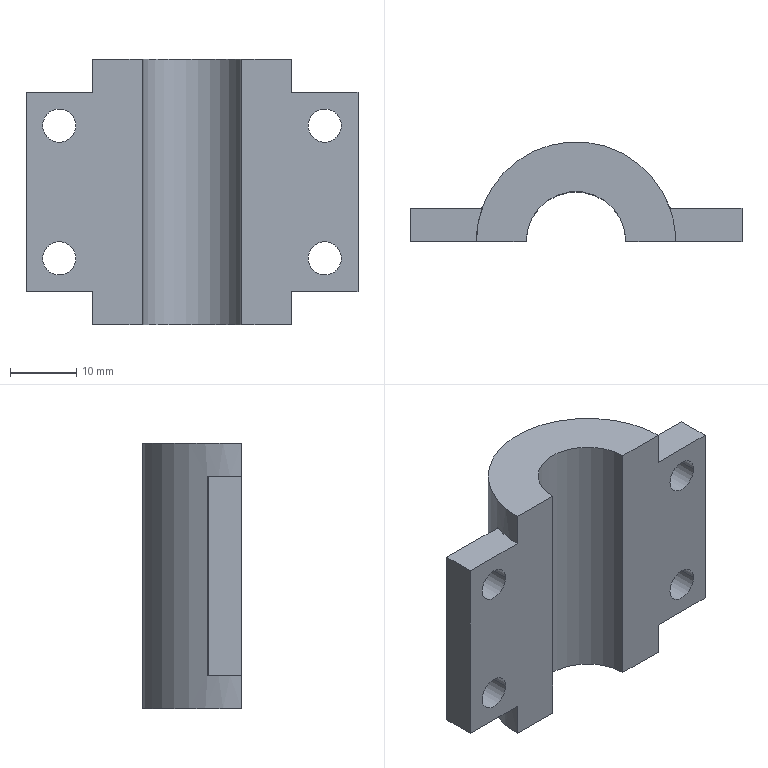Part | SolidWorks | features BaseBody 1 | 1 solid | 28 faces | box 50 x 15 x 40 mm | volume 13295 mm3 | cylinder 16 | plane 12 | commonest cylinder face diameters 5 x8 0.5 x4 30 x3 15 x1
STEP:
#1=CARTESIAN_POINT('',(-17.5,0.,10.));
#2=VERTEX_POINT('',#1);
#3=CARTESIAN_POINT('',(-22.5,0.,10.));
#4=VERTEX_POINT('',#3);
#5=CARTESIAN_POINT('',(-20.,0.,10.));
#6=DIRECTION('',(0.,1.,0.));
#7=DIRECTION('',(-1.,0.,0.));
#8=AXIS2_PLACEMENT_3D('',#5,#6,#7);
#9=CIRCLE('',#8,2.5);
#10=EDGE_CURVE('',#2,#4,#9,.T.);
#11=ORIENTED_EDGE('',*,*,#10,.F.);
#12=CARTESIAN_POINT('',(-17.5,5.,10.));
#13=VERTEX_POINT('',#12);
#14=CARTESIAN_POINT('',(-17.5,5.,10.));
#15=DIRECTION('',(0.,1.,0.));
#16=VECTOR('',#15,1000.);
#17=LINE('',#14,#16);
#18=EDGE_CURVE('',#2,#13,#17,.T.);
#19=ORIENTED_EDGE('',*,*,#18,.T.);
#20=CARTESIAN_POINT('',(-22.5,5.,10.));
#21=VERTEX_POINT('',#20);
#22=CARTESIAN_POINT('',(-20.,5.,10.));
#23=DIRECTION('',(0.,-1.,0.));
#24=DIRECTION('',(-1.,0.,0.));
#25=AXIS2_PLACEMENT_3D('',#22,#23,#24);
#26=CIRCLE('',#25,2.5);
#27=EDGE_CURVE('',#21,#13,#26,.T.);
#28=ORIENTED_EDGE('',*,*,#27,.F.);
#29=CARTESIAN_POINT('',(-22.5,5.,10.));
#30=DIRECTION('',(0.,1.,0.));
#31=VECTOR('',#30,1000.);
#32=LINE('',#29,#31);
#33=EDGE_CURVE('',#4,#21,#32,.T.);
#34=ORIENTED_EDGE('',*,*,#33,.F.);
#35=EDGE_LOOP('',(#11,#19,#28,#34));
#36=FACE_OUTER_BOUND('',#35,.T.);
#37=CARTESIAN_POINT('',(-20.,5.,10.));
#38=DIRECTION('',(0.,1.,0.));
#39=DIRECTION('',(-1.,0.,0.));
#40=AXIS2_PLACEMENT_3D('',#37,#38,#39);
#41=CYLINDRICAL_SURFACE('',#40,2.5);
#42=ADVANCED_FACE('',(#36),#41,.F.);
#43=CARTESIAN_POINT('',(22.5,0.,10.));
#44=VERTEX_POINT('',#43);
#45=CARTESIAN_POINT('',(17.5,0.,10.));
#46=VERTEX_POINT('',#45);
#47=CARTESIAN_POINT('',(20.,0.,10.));
#48=DIRECTION('',(0.,1.,0.));
#49=DIRECTION('',(-1.,0.,0.));
#50=AXIS2_PLACEMENT_3D('',#47,#48,#49);
#51=CIRCLE('',#50,2.5);
#52=EDGE_CURVE('',#44,#46,#51,.T.);
#53=ORIENTED_EDGE('',*,*,#52,.F.);
#54=CARTESIAN_POINT('',(22.5,5.,10.));
#55=VERTEX_POINT('',#54);
#56=CARTESIAN_POINT('',(22.5,5.,10.));
#57=DIRECTION('',(0.,1.,0.));
#58=VECTOR('',#57,1000.);
#59=LINE('',#56,#58);
#60=EDGE_CURVE('',#44,#55,#59,.T.);
#61=ORIENTED_EDGE('',*,*,#60,.T.);
#62=CARTESIAN_POINT('',(17.5,5.,10.));
#63=VERTEX_POINT('',#62);
#64=CARTESIAN_POINT('',(20.,5.,10.));
#65=DIRECTION('',(0.,-1.,0.));
#66=DIRECTION('',(-1.,0.,0.));
#67=AXIS2_PLACEMENT_3D('',#64,#65,#66);
#68=CIRCLE('',#67,2.5);
#69=EDGE_CURVE('',#63,#55,#68,.T.);
#70=ORIENTED_EDGE('',*,*,#69,.F.);
#71=CARTESIAN_POINT('',(17.5,5.,10.));
#72=DIRECTION('',(0.,1.,0.));
#73=VECTOR('',#72,1000.);
#74=LINE('',#71,#73);
#75=EDGE_CURVE('',#46,#63,#74,.T.);
#76=ORIENTED_EDGE('',*,*,#75,.F.);
#77=EDGE_LOOP('',(#53,#61,#70,#76));
#78=FACE_OUTER_BOUND('',#77,.T.);
#79=CARTESIAN_POINT('',(20.,5.,10.));
#80=DIRECTION('',(0.,1.,0.));
#81=DIRECTION('',(-1.,0.,0.));
#82=AXIS2_PLACEMENT_3D('',#79,#80,#81);
#83=CYLINDRICAL_SURFACE('',#82,2.5);
#84=ADVANCED_FACE('',(#78),#83,.F.);
#85=CARTESIAN_POINT('',(22.5,0.,30.));
#86=VERTEX_POINT('',#85);
#87=CARTESIAN_POINT('',(17.5,0.,30.));
#88=VERTEX_POINT('',#87);
#89=CARTESIAN_POINT('',(20.,0.,30.));
#90=DIRECTION('',(0.,1.,0.));
#91=DIRECTION('',(-1.,0.,0.));
#92=AXIS2_PLACEMENT_3D('',#89,#90,#91);
#93=CIRCLE('',#92,2.5);
#94=EDGE_CURVE('',#86,#88,#93,.T.);
#95=ORIENTED_EDGE('',*,*,#94,.F.);
#96=CARTESIAN_POINT('',(22.5,5.,30.));
#97=VERTEX_POINT('',#96);
#98=CARTESIAN_POINT('',(22.5,5.,30.));
#99=DIRECTION('',(0.,1.,0.));
#100=VECTOR('',#99,1000.);
#101=LINE('',#98,#100);
#102=EDGE_CURVE('',#86,#97,#101,.T.);
#103=ORIENTED_EDGE('',*,*,#102,.T.);
#104=CARTESIAN_POINT('',(17.5,5.,30.));
#105=VERTEX_POINT('',#104);
#106=CARTESIAN_POINT('',(20.,5.,30.));
#107=DIRECTION('',(0.,-1.,0.));
#108=DIRECTION('',(-1.,0.,0.));
#109=AXIS2_PLACEMENT_3D('',#106,#107,#108);
#110=CIRCLE('',#109,2.5);
#111=EDGE_CURVE('',#105,#97,#110,.T.);
#112=ORIENTED_EDGE('',*,*,#111,.F.);
#113=CARTESIAN_POINT('',(17.5,5.,30.));
#114=DIRECTION('',(0.,1.,0.));
#115=VECTOR('',#114,1000.);
#116=LINE('',#113,#115);
#117=EDGE_CURVE('',#88,#105,#116,.T.);
#118=ORIENTED_EDGE('',*,*,#117,.F.);
#119=EDGE_LOOP('',(#95,#103,#112,#118));
#120=FACE_OUTER_BOUND('',#119,.T.);
#121=CARTESIAN_POINT('',(20.,5.,30.));
#122=DIRECTION('',(0.,1.,0.));
#123=DIRECTION('',(-1.,0.,0.));
#124=AXIS2_PLACEMENT_3D('',#121,#122,#123);
#125=CYLINDRICAL_SURFACE('',#124,2.5);
#126=ADVANCED_FACE('',(#120),#125,.F.);
#127=CARTESIAN_POINT('',(-17.5,0.,30.));
#128=VERTEX_POINT('',#127);
#129=CARTESIAN_POINT('',(-22.5,0.,30.));
#130=VERTEX_POINT('',#129);
#131=CARTESIAN_POINT('',(-20.,0.,30.));
#132=DIRECTION('',(0.,1.,0.));
#133=DIRECTION('',(-1.,0.,0.));
#134=AXIS2_PLACEMENT_3D('',#131,#132,#133);
#135=CIRCLE('',#134,2.5);
#136=EDGE_CURVE('',#128,#130,#135,.T.);
#137=ORIENTED_EDGE('',*,*,#136,.F.);
#138=CARTESIAN_POINT('',(-17.5,5.,30.));
#139=VERTEX_POINT('',#138);
#140=CARTESIAN_POINT('',(-17.5,5.,30.));
#141=DIRECTION('',(0.,1.,0.));
#142=VECTOR('',#141,1000.);
#143=LINE('',#140,#142);
#144=EDGE_CURVE('',#128,#139,#143,.T.);
#145=ORIENTED_EDGE('',*,*,#144,.T.);
#146=CARTESIAN_POINT('',(-22.5,5.,30.));
#147=VERTEX_POINT('',#146);
#148=CARTESIAN_POINT('',(-20.,5.,30.));
#149=DIRECTION('',(0.,-1.,0.));
#150=DIRECTION('',(-1.,0.,0.));
#151=AXIS2_PLACEMENT_3D('',#148,#149,#150);
#152=CIRCLE('',#151,2.5);
#153=EDGE_CURVE('',#147,#139,#152,.T.);
#154=ORIENTED_EDGE('',*,*,#153,.F.);
#155=CARTESIAN_POINT('',(-22.5,5.,30.));
#156=DIRECTION('',(0.,1.,0.));
#157=VECTOR('',#156,1000.);
#158=LINE('',#155,#157);
#159=EDGE_CURVE('',#130,#147,#158,.T.);
#160=ORIENTED_EDGE('',*,*,#159,.F.);
#161=EDGE_LOOP('',(#137,#145,#154,#160));
#162=FACE_OUTER_BOUND('',#161,.T.);
#163=CARTESIAN_POINT('',(-20.,5.,30.));
#164=DIRECTION('',(0.,1.,0.));
#165=DIRECTION('',(-1.,0.,0.));
#166=AXIS2_PLACEMENT_3D('',#163,#164,#165);
#167=CYLINDRICAL_SURFACE('',#166,2.5);
#168=ADVANCED_FACE('',(#162),#167,.F.);
#169=CARTESIAN_POINT('',(-14.083,5.164,5.));
#170=VERTEX_POINT('',#169);
#171=CARTESIAN_POINT('',(-14.175,5.045,5.));
#172=VERTEX_POINT('',#171);
#173=CARTESIAN_POINT('',(-14.318,5.25,5.));
#174=DIRECTION('',(0.,0.,-1.));
#175=DIRECTION('',(0.5726,-0.8198,0.));
#176=AXIS2_PLACEMENT_3D('',#173,#174,#175);
#177=CIRCLE('',#176,0.25);
#178=EDGE_CURVE('',#170,#172,#177,.T.);
#179=ORIENTED_EDGE('',*,*,#178,.T.);
#180=CARTESIAN_POINT('',(-14.175,5.045,35.));
#181=VERTEX_POINT('',#180);
#182=CARTESIAN_POINT('',(-14.175,5.045,0.));
#183=DIRECTION('',(0.,0.,1.));
#184=VECTOR('',#183,1000.);
#185=LINE('',#182,#184);
#186=EDGE_CURVE('',#172,#181,#185,.T.);
#187=ORIENTED_EDGE('',*,*,#186,.T.);
#188=CARTESIAN_POINT('',(-14.083,5.164,35.));
#189=VERTEX_POINT('',#188);
#190=CARTESIAN_POINT('',(-14.318,5.25,35.));
#191=DIRECTION('',(0.,0.,1.));
#192=DIRECTION('',(0.5726,-0.8198,0.));
#193=AXIS2_PLACEMENT_3D('',#190,#191,#192);
#194=CIRCLE('',#193,0.25);
#195=EDGE_CURVE('',#181,#189,#194,.T.);
#196=ORIENTED_EDGE('',*,*,#195,.T.);
#197=CARTESIAN_POINT('',(-14.083,5.164,0.));
#198=DIRECTION('',(0.,0.,-1.));
#199=VECTOR('',#198,1000.);
#200=LINE('',#197,#199);
#201=EDGE_CURVE('',#189,#170,#200,.T.);
#202=ORIENTED_EDGE('',*,*,#201,.T.);
#203=EDGE_LOOP('',(#179,#187,#196,#202));
#204=FACE_OUTER_BOUND('',#203,.T.);
#205=CARTESIAN_POINT('',(-14.318,5.25,0.));
#206=DIRECTION('',(0.,0.,1.));
#207=DIRECTION('',(0.5726,-0.8198,0.));
#208=AXIS2_PLACEMENT_3D('',#205,#206,#207);
#209=CYLINDRICAL_SURFACE('',#208,0.25);
#210=ADVANCED_FACE('',(#204),#209,.F.);
#211=CARTESIAN_POINT('',(14.142,5.,40.));
#212=VERTEX_POINT('',#211);
#213=CARTESIAN_POINT('',(-15.,0.,40.));
#214=VERTEX_POINT('',#213);
#215=CARTESIAN_POINT('',(0.,0.,40.));
#216=DIRECTION('',(0.,0.,1.));
#217=DIRECTION('',(0.9428,-0.3333,0.));
#218=AXIS2_PLACEMENT_3D('',#215,#216,#217);
#219=CIRCLE('',#218,15.);
#220=EDGE_CURVE('',#212,#214,#219,.T.);
#221=ORIENTED_EDGE('',*,*,#220,.F.);
#222=CARTESIAN_POINT('',(14.142,5.,35.));
#223=VERTEX_POINT('',#222);
#224=CARTESIAN_POINT('',(14.142,5.,0.));
#225=DIRECTION('',(0.,0.,-1.));
#226=VECTOR('',#225,1000.);
#227=LINE('',#224,#226);
#228=EDGE_CURVE('',#212,#223,#227,.T.);
#229=ORIENTED_EDGE('',*,*,#228,.T.);
#230=CARTESIAN_POINT('',(14.083,5.164,35.));
#231=VERTEX_POINT('',#230);
#232=CARTESIAN_POINT('',(0.,0.,35.));
#233=DIRECTION('',(0.,0.,1.));
#234=DIRECTION('',(0.9428,0.3333,0.));
#235=AXIS2_PLACEMENT_3D('',#232,#233,#234);
#236=CIRCLE('',#235,15.);
#237=EDGE_CURVE('',#223,#231,#236,.T.);
#238=ORIENTED_EDGE('',*,*,#237,.T.);
#239=CARTESIAN_POINT('',(14.083,5.164,5.));
#240=VERTEX_POINT('',#239);
#241=CARTESIAN_POINT('',(14.083,5.164,0.));
#242=DIRECTION('',(0.,0.,1.));
#243=VECTOR('',#242,1000.);
#244=LINE('',#241,#243);
#245=EDGE_CURVE('',#240,#231,#244,.T.);
#246=ORIENTED_EDGE('',*,*,#245,.F.);
#247=CARTESIAN_POINT('',(14.142,5.,5.));
#248=VERTEX_POINT('',#247);
#249=CARTESIAN_POINT('',(0.,0.,5.));
#250=DIRECTION('',(0.,0.,-1.));
#251=DIRECTION('',(0.9428,0.3333,0.));
#252=AXIS2_PLACEMENT_3D('',#249,#250,#251);
#253=CIRCLE('',#252,15.);
#254=EDGE_CURVE('',#240,#248,#253,.T.);
#255=ORIENTED_EDGE('',*,*,#254,.T.);
#256=CARTESIAN_POINT('',(14.142,5.,0.));
#257=VERTEX_POINT('',#256);
#258=CARTESIAN_POINT('',(14.142,5.,0.));
#259=DIRECTION('',(0.,0.,-1.));
#260=VECTOR('',#259,1000.);
#261=LINE('',#258,#260);
#262=EDGE_CURVE('',#248,#257,#261,.T.);
#263=ORIENTED_EDGE('',*,*,#262,.T.);
#264=CARTESIAN_POINT('',(-15.,0.,0.));
#265=VERTEX_POINT('',#264);
#266=CARTESIAN_POINT('',(0.,0.,0.));
#267=DIRECTION('',(0.,0.,-1.));
#268=DIRECTION('',(-1.,0.,0.));
#269=AXIS2_PLACEMENT_3D('',#266,#267,#268);
#270=CIRCLE('',#269,15.);
#271=EDGE_CURVE('',#265,#257,#270,.T.);
#272=ORIENTED_EDGE('',*,*,#271,.F.);
#273=CARTESIAN_POINT('',(-15.,0.,5.));
#274=VERTEX_POINT('',#273);
#275=CARTESIAN_POINT('',(-15.,0.,5.));
#276=DIRECTION('',(0.,0.,-1.));
#277=VECTOR('',#276,1000.);
#278=LINE('',#275,#277);
#279=EDGE_CURVE('',#274,#265,#278,.T.);
#280=ORIENTED_EDGE('',*,*,#279,.F.);
#281=CARTESIAN_POINT('',(0.,0.,5.));
#282=DIRECTION('',(0.,0.,-1.));
#283=DIRECTION('',(0.9428,0.3333,0.));
#284=AXIS2_PLACEMENT_3D('',#281,#282,#283);
#285=CIRCLE('',#284,15.);
#286=EDGE_CURVE('',#274,#170,#285,.T.);
#287=ORIENTED_EDGE('',*,*,#286,.T.);
#288=ORIENTED_EDGE('',*,*,#201,.F.);
#289=CARTESIAN_POINT('',(-15.,0.,35.));
#290=VERTEX_POINT('',#289);
#291=CARTESIAN_POINT('',(0.,0.,35.));
#292=DIRECTION('',(0.,0.,1.));
#293=DIRECTION('',(0.9428,0.3333,0.));
#294=AXIS2_PLACEMENT_3D('',#291,#292,#293);
#295=CIRCLE('',#294,15.);
#296=EDGE_CURVE('',#189,#290,#295,.T.);
#297=ORIENTED_EDGE('',*,*,#296,.T.);
#298=CARTESIAN_POINT('',(-15.,0.,40.));
#299=DIRECTION('',(0.,0.,-1.));
#300=VECTOR('',#299,1000.);
#301=LINE('',#298,#300);
#302=EDGE_CURVE('',#214,#290,#301,.T.);
#303=ORIENTED_EDGE('',*,*,#302,.F.);
#304=EDGE_LOOP('',(#221,#229,#238,#246,#255,#263,#272,#280,#287,#288,#297,#303));
#305=FACE_OUTER_BOUND('',#304,.T.);
#306=CARTESIAN_POINT('',(0.,0.,0.));
#307=DIRECTION('',(0.,0.,-1.));
#308=DIRECTION('',(0.9428,0.3333,0.));
#309=AXIS2_PLACEMENT_3D('',#306,#307,#308);
#310=CYLINDRICAL_SURFACE('',#309,15.);
#311=ADVANCED_FACE('',(#305),#310,.T.);
#312=ORIENTED_EDGE('',*,*,#228,.F.);
#313=CARTESIAN_POINT('',(15.,0.,40.));
#314=VERTEX_POINT('',#313);
#315=CARTESIAN_POINT('',(0.,0.,40.));
#316=DIRECTION('',(0.,0.,1.));
#317=DIRECTION('',(0.9428,-0.3333,0.));
#318=AXIS2_PLACEMENT_3D('',#315,#316,#317);
#319=CIRCLE('',#318,15.);
#320=EDGE_CURVE('',#314,#212,#319,.T.);
#321=ORIENTED_EDGE('',*,*,#320,.F.);
#322=CARTESIAN_POINT('',(15.,0.,35.));
#323=VERTEX_POINT('',#322);
#324=CARTESIAN_POINT('',(15.,0.,40.));
#325=DIRECTION('',(0.,0.,1.));
#326=VECTOR('',#325,1000.);
#327=LINE('',#324,#326);
#328=EDGE_CURVE('',#323,#314,#327,.T.);
#329=ORIENTED_EDGE('',*,*,#328,.F.);
#330=CARTESIAN_POINT('',(0.,0.,35.));
#331=DIRECTION('',(0.,0.,1.));
#332=DIRECTION('',(0.9428,0.3333,0.));
#333=AXIS2_PLACEMENT_3D('',#330,#331,#332);
#334=CIRCLE('',#333,15.);
#335=EDGE_CURVE('',#323,#223,#334,.T.);
#336=ORIENTED_EDGE('',*,*,#335,.T.);
#337=EDGE_LOOP('',(#312,#321,#329,#336));
#338=FACE_OUTER_BOUND('',#337,.T.);
#339=CARTESIAN_POINT('',(0.,0.,0.));
#340=DIRECTION('',(0.,0.,-1.));
#341=DIRECTION('',(0.9428,0.3333,0.));
#342=AXIS2_PLACEMENT_3D('',#339,#340,#341);
#343=CYLINDRICAL_SURFACE('',#342,15.);
#344=ADVANCED_FACE('',(#338),#343,.T.);
#345=CARTESIAN_POINT('',(14.175,5.045,35.));
#346=VERTEX_POINT('',#345);
#347=CARTESIAN_POINT('',(14.318,5.25,35.));
#348=DIRECTION('',(0.,0.,1.));
#349=DIRECTION('',(-0.5726,-0.8198,0.));
#350=AXIS2_PLACEMENT_3D('',#347,#348,#349);
#351=CIRCLE('',#350,0.25);
#352=EDGE_CURVE('',#231,#346,#351,.T.);
#353=ORIENTED_EDGE('',*,*,#352,.T.);
#354=CARTESIAN_POINT('',(14.175,5.045,5.));
#355=VERTEX_POINT('',#354);
#356=CARTESIAN_POINT('',(14.175,5.045,0.));
#357=DIRECTION('',(0.,0.,-1.));
#358=VECTOR('',#357,1000.);
#359=LINE('',#356,#358);
#360=EDGE_CURVE('',#346,#355,#359,.T.);
#361=ORIENTED_EDGE('',*,*,#360,.T.);
#362=CARTESIAN_POINT('',(14.318,5.25,5.));
#363=DIRECTION('',(0.,0.,-1.));
#364=DIRECTION('',(-0.5726,-0.8198,0.));
#365=AXIS2_PLACEMENT_3D('',#362,#363,#364);
#366=CIRCLE('',#365,0.25);
#367=EDGE_CURVE('',#355,#240,#366,.T.);
#368=ORIENTED_EDGE('',*,*,#367,.T.);
#369=ORIENTED_EDGE('',*,*,#245,.T.);
#370=EDGE_LOOP('',(#353,#361,#368,#369));
#371=FACE_OUTER_BOUND('',#370,.T.);
#372=CARTESIAN_POINT('',(14.318,5.25,0.));
#373=DIRECTION('',(0.,0.,-1.));
#374=DIRECTION('',(-0.5726,-0.8198,0.));
#375=AXIS2_PLACEMENT_3D('',#372,#373,#374);
#376=CYLINDRICAL_SURFACE('',#375,0.25);
#377=ADVANCED_FACE('',(#371),#376,.F.);
#378=ORIENTED_EDGE('',*,*,#254,.F.);
#379=ORIENTED_EDGE('',*,*,#367,.F.);
#380=CARTESIAN_POINT('',(14.318,5.,5.));
#381=VERTEX_POINT('',#380);
#382=CARTESIAN_POINT('',(14.318,5.25,5.));
#383=DIRECTION('',(0.,0.,-1.));
#384=DIRECTION('',(-0.5726,-0.8198,0.));
#385=AXIS2_PLACEMENT_3D('',#382,#383,#384);
#386=CIRCLE('',#385,0.25);
#387=EDGE_CURVE('',#381,#355,#386,.T.);
#388=ORIENTED_EDGE('',*,*,#387,.F.);
#389=CARTESIAN_POINT('',(25.,5.,5.));
#390=VERTEX_POINT('',#389);
#391=CARTESIAN_POINT('',(17.073,5.,5.));
#392=DIRECTION('',(-1.,0.,0.));
#393=VECTOR('',#392,1000.);
#394=LINE('',#391,#393);
#395=EDGE_CURVE('',#390,#381,#394,.T.);
#396=ORIENTED_EDGE('',*,*,#395,.F.);
#397=CARTESIAN_POINT('',(25.,0.,5.));
#398=VERTEX_POINT('',#397);
#399=CARTESIAN_POINT('',(25.,1.288,5.));
#400=DIRECTION('',(0.,1.,0.));
#401=VECTOR('',#400,1000.);
#402=LINE('',#399,#401);
#403=EDGE_CURVE('',#398,#390,#402,.T.);
#404=ORIENTED_EDGE('',*,*,#403,.F.);
#405=CARTESIAN_POINT('',(15.,0.,5.));
#406=VERTEX_POINT('',#405);
#407=CARTESIAN_POINT('',(13.752,0.,5.));
#408=DIRECTION('',(1.,0.,0.));
#409=VECTOR('',#408,1000.);
#410=LINE('',#407,#409);
#411=EDGE_CURVE('',#406,#398,#410,.T.);
#412=ORIENTED_EDGE('',*,*,#411,.F.);
#413=CARTESIAN_POINT('',(0.,0.,5.));
#414=DIRECTION('',(0.,0.,-1.));
#415=DIRECTION('',(0.9428,0.3333,0.));
#416=AXIS2_PLACEMENT_3D('',#413,#414,#415);
#417=CIRCLE('',#416,15.);
#418=EDGE_CURVE('',#248,#406,#417,.T.);
#419=ORIENTED_EDGE('',*,*,#418,.F.);
#420=EDGE_LOOP('',(#378,#379,#388,#396,#404,#412,#419));
#421=FACE_OUTER_BOUND('',#420,.T.);
#422=CARTESIAN_POINT('',(20.004,2.575,5.));
#423=DIRECTION('',(0.,0.,1.));
#424=DIRECTION('',(1.,0.,0.));
#425=AXIS2_PLACEMENT_3D('',#422,#423,#424);
#426=PLANE('',#425);
#427=ADVANCED_FACE('',(#421),#426,.F.);
#428=ORIENTED_EDGE('',*,*,#286,.F.);
#429=CARTESIAN_POINT('',(-25.,0.,5.));
#430=VERTEX_POINT('',#429);
#431=CARTESIAN_POINT('',(-17.502,0.,5.));
#432=DIRECTION('',(1.,0.,0.));
#433=VECTOR('',#432,1000.);
#434=LINE('',#431,#433);
#435=EDGE_CURVE('',#430,#274,#434,.T.);
#436=ORIENTED_EDGE('',*,*,#435,.F.);
#437=CARTESIAN_POINT('',(-25.,5.,5.));
#438=VERTEX_POINT('',#437);
#439=CARTESIAN_POINT('',(-25.,3.788,5.));
#440=DIRECTION('',(0.,-1.,0.));
#441=VECTOR('',#440,1000.);
#442=LINE('',#439,#441);
#443=EDGE_CURVE('',#438,#430,#442,.T.);
#444=ORIENTED_EDGE('',*,*,#443,.F.);
#445=CARTESIAN_POINT('',(-14.318,5.,5.));
#446=VERTEX_POINT('',#445);
#447=CARTESIAN_POINT('',(-12.797,5.,5.));
#448=DIRECTION('',(-1.,0.,0.));
#449=VECTOR('',#448,1000.);
#450=LINE('',#447,#449);
#451=EDGE_CURVE('',#446,#438,#450,.T.);
#452=ORIENTED_EDGE('',*,*,#451,.F.);
#453=CARTESIAN_POINT('',(-14.318,5.25,5.));
#454=DIRECTION('',(0.,0.,-1.));
#455=DIRECTION('',(0.5726,-0.8198,0.));
#456=AXIS2_PLACEMENT_3D('',#453,#454,#455);
#457=CIRCLE('',#456,0.25);
#458=EDGE_CURVE('',#172,#446,#457,.T.);
#459=ORIENTED_EDGE('',*,*,#458,.F.);
#460=ORIENTED_EDGE('',*,*,#178,.F.);
#461=EDGE_LOOP('',(#428,#436,#444,#452,#459,#460));
#462=FACE_OUTER_BOUND('',#461,.T.);
#463=CARTESIAN_POINT('',(-20.004,2.575,5.));
#464=DIRECTION('',(0.,0.,1.));
#465=DIRECTION('',(1.,0.,0.));
#466=AXIS2_PLACEMENT_3D('',#463,#464,#465);
#467=PLANE('',#466);
#468=ADVANCED_FACE('',(#462),#467,.F.);
#469=ORIENTED_EDGE('',*,*,#403,.T.);
#470=CARTESIAN_POINT('',(25.,5.,35.));
#471=VERTEX_POINT('',#470);
#472=CARTESIAN_POINT('',(25.,5.,0.));
#473=DIRECTION('',(0.,0.,1.));
#474=VECTOR('',#473,1000.);
#475=LINE('',#472,#474);
#476=EDGE_CURVE('',#390,#471,#475,.T.);
#477=ORIENTED_EDGE('',*,*,#476,.T.);
#478=CARTESIAN_POINT('',(25.,0.,35.));
#479=VERTEX_POINT('',#478);
#480=CARTESIAN_POINT('',(25.,1.288,35.));
#481=DIRECTION('',(0.,-1.,0.));
#482=VECTOR('',#481,1000.);
#483=LINE('',#480,#482);
#484=EDGE_CURVE('',#471,#479,#483,.T.);
#485=ORIENTED_EDGE('',*,*,#484,.T.);
#486=CARTESIAN_POINT('',(25.,0.,0.));
#487=DIRECTION('',(0.,0.,1.));
#488=VECTOR('',#487,1000.);
#489=LINE('',#486,#488);
#490=EDGE_CURVE('',#398,#479,#489,.T.);
#491=ORIENTED_EDGE('',*,*,#490,.F.);
#492=EDGE_LOOP('',(#469,#477,#485,#491));
#493=FACE_OUTER_BOUND('',#492,.T.);
#494=CARTESIAN_POINT('',(25.,0.,0.));
#495=DIRECTION('',(1.,0.,0.));
#496=DIRECTION('',(0.,1.,0.));
#497=AXIS2_PLACEMENT_3D('',#494,#495,#496);
#498=PLANE('',#497);
#499=ADVANCED_FACE('',(#493),#498,.T.);
#500=ORIENTED_EDGE('',*,*,#69,.T.);
#501=CARTESIAN_POINT('',(20.,5.,10.));
#502=DIRECTION('',(0.,-1.,0.));
#503=DIRECTION('',(-1.,0.,0.));
#504=AXIS2_PLACEMENT_3D('',#501,#502,#503);
#505=CIRCLE('',#504,2.5);
#506=EDGE_CURVE('',#55,#63,#505,.T.);
#507=ORIENTED_EDGE('',*,*,#506,.T.);
#508=EDGE_LOOP('',(#500,#507));
#509=FACE_BOUND('',#508,.T.);
#510=ORIENTED_EDGE('',*,*,#111,.T.);
#511=CARTESIAN_POINT('',(20.,5.,30.));
#512=DIRECTION('',(0.,-1.,0.));
#513=DIRECTION('',(-1.,0.,0.));
#514=AXIS2_PLACEMENT_3D('',#511,#512,#513);
#515=CIRCLE('',#514,2.5);
#516=EDGE_CURVE('',#97,#105,#515,.T.);
#517=ORIENTED_EDGE('',*,*,#516,.T.);
#518=EDGE_LOOP('',(#510,#517));
#519=FACE_BOUND('',#518,.T.);
#520=CARTESIAN_POINT('',(14.318,5.,35.));
#521=VERTEX_POINT('',#520);
#522=CARTESIAN_POINT('',(14.318,5.,0.));
#523=DIRECTION('',(0.,0.,-1.));
#524=VECTOR('',#523,1000.);
#525=LINE('',#522,#524);
#526=EDGE_CURVE('',#521,#381,#525,.T.);
#527=ORIENTED_EDGE('',*,*,#526,.F.);
#528=CARTESIAN_POINT('',(17.073,5.,35.));
#529=DIRECTION('',(1.,0.,0.));
#530=VECTOR('',#529,1000.);
#531=LINE('',#528,#530);
#532=EDGE_CURVE('',#521,#471,#531,.T.);
#533=ORIENTED_EDGE('',*,*,#532,.T.);
#534=ORIENTED_EDGE('',*,*,#476,.F.);
#535=ORIENTED_EDGE('',*,*,#395,.T.);
#536=EDGE_LOOP('',(#527,#533,#534,#535));
#537=FACE_OUTER_BOUND('',#536,.T.);
#538=CARTESIAN_POINT('',(14.142,5.,0.));
#539=DIRECTION('',(0.,1.,0.));
#540=DIRECTION('',(1.,0.,0.));
#541=AXIS2_PLACEMENT_3D('',#538,#539,#540);
#542=PLANE('',#541);
#543=ADVANCED_FACE('',(#509,#519,#537),#542,.T.);
#544=CARTESIAN_POINT('',(-20.,0.,10.));
#545=DIRECTION('',(0.,1.,0.));
#546=DIRECTION('',(-1.,0.,0.));
#547=AXIS2_PLACEMENT_3D('',#544,#545,#546);
#548=CIRCLE('',#547,2.5);
#549=EDGE_CURVE('',#4,#2,#548,.T.);
#550=ORIENTED_EDGE('',*,*,#549,.T.);
#551=ORIENTED_EDGE('',*,*,#10,.T.);
#552=EDGE_LOOP('',(#550,#551));
#553=FACE_BOUND('',#552,.T.);
#554=CARTESIAN_POINT('',(-20.,0.,30.));
#555=DIRECTION('',(0.,1.,0.));
#556=DIRECTION('',(-1.,0.,0.));
#557=AXIS2_PLACEMENT_3D('',#554,#555,#556);
#558=CIRCLE('',#557,2.5);
#559=EDGE_CURVE('',#130,#128,#558,.T.);
#560=ORIENTED_EDGE('',*,*,#559,.T.);
#561=ORIENTED_EDGE('',*,*,#136,.T.);
#562=EDGE_LOOP('',(#560,#561));
#563=FACE_BOUND('',#562,.T.);
#564=ORIENTED_EDGE('',*,*,#435,.T.);
#565=ORIENTED_EDGE('',*,*,#279,.T.);
#566=CARTESIAN_POINT('',(-7.5,0.,0.));
#567=VERTEX_POINT('',#566);
#568=CARTESIAN_POINT('',(-25.,0.,0.));
#569=DIRECTION('',(1.,0.,0.));
#570=VECTOR('',#569,1000.);
#571=LINE('',#568,#570);
#572=EDGE_CURVE('',#265,#567,#571,.T.);
#573=ORIENTED_EDGE('',*,*,#572,.T.);
#574=CARTESIAN_POINT('',(-7.5,0.,40.));
#575=VERTEX_POINT('',#574);
#576=CARTESIAN_POINT('',(-7.5,0.,0.));
#577=DIRECTION('',(0.,0.,1.));
#578=VECTOR('',#577,1000.);
#579=LINE('',#576,#578);
#580=EDGE_CURVE('',#567,#575,#579,.T.);
#581=ORIENTED_EDGE('',*,*,#580,.T.);
#582=CARTESIAN_POINT('',(-25.,0.,40.));
#583=DIRECTION('',(1.,0.,0.));
#584=VECTOR('',#583,1000.);
#585=LINE('',#582,#584);
#586=EDGE_CURVE('',#214,#575,#585,.T.);
#587=ORIENTED_EDGE('',*,*,#586,.F.);
#588=ORIENTED_EDGE('',*,*,#302,.T.);
#589=CARTESIAN_POINT('',(-25.,0.,35.));
#590=VERTEX_POINT('',#589);
#591=CARTESIAN_POINT('',(-17.502,0.,35.));
#592=DIRECTION('',(-1.,0.,0.));
#593=VECTOR('',#592,1000.);
#594=LINE('',#591,#593);
#595=EDGE_CURVE('',#290,#590,#594,.T.);
#596=ORIENTED_EDGE('',*,*,#595,.T.);
#597=CARTESIAN_POINT('',(-25.,0.,0.));
#598=DIRECTION('',(0.,0.,1.));
#599=VECTOR('',#598,1000.);
#600=LINE('',#597,#599);
#601=EDGE_CURVE('',#430,#590,#600,.T.);
#602=ORIENTED_EDGE('',*,*,#601,.F.);
#603=EDGE_LOOP('',(#564,#565,#573,#581,#587,#588,#596,#602));
#604=FACE_OUTER_BOUND('',#603,.T.);
#605=CARTESIAN_POINT('',(-15.,0.,0.));
#606=DIRECTION('',(0.,-1.,0.));
#607=DIRECTION('',(0.,0.,-1.));
#608=AXIS2_PLACEMENT_3D('',#605,#606,#607);
#609=PLANE('',#608);
#610=ADVANCED_FACE('',(#553,#563,#604),#609,.T.);
#611=ORIENTED_EDGE('',*,*,#335,.F.);
#612=CARTESIAN_POINT('',(13.752,0.,35.));
#613=DIRECTION('',(-1.,0.,0.));
#614=VECTOR('',#613,1000.);
#615=LINE('',#612,#614);
#616=EDGE_CURVE('',#479,#323,#615,.T.);
#617=ORIENTED_EDGE('',*,*,#616,.F.);
#618=ORIENTED_EDGE('',*,*,#484,.F.);
#619=ORIENTED_EDGE('',*,*,#532,.F.);
#620=CARTESIAN_POINT('',(14.318,5.25,35.));
#621=DIRECTION('',(0.,0.,1.));
#622=DIRECTION('',(-0.5726,-0.8198,0.));
#623=AXIS2_PLACEMENT_3D('',#620,#621,#622);
#624=CIRCLE('',#623,0.25);
#625=EDGE_CURVE('',#346,#521,#624,.T.);
#626=ORIENTED_EDGE('',*,*,#625,.F.);
#627=ORIENTED_EDGE('',*,*,#352,.F.);
#628=ORIENTED_EDGE('',*,*,#237,.F.);
#629=EDGE_LOOP('',(#611,#617,#618,#619,#626,#627,#628));
#630=FACE_OUTER_BOUND('',#629,.T.);
#631=CARTESIAN_POINT('',(20.004,2.575,35.));
#632=DIRECTION('',(0.,0.,1.));
#633=DIRECTION('',(1.,0.,0.));
#634=AXIS2_PLACEMENT_3D('',#631,#632,#633);
#635=PLANE('',#634);
#636=ADVANCED_FACE('',(#630),#635,.T.);
#637=CARTESIAN_POINT('',(-25.,5.,35.));
#638=VERTEX_POINT('',#637);
#639=CARTESIAN_POINT('',(-14.318,5.,35.));
#640=VERTEX_POINT('',#639);
#641=CARTESIAN_POINT('',(-12.797,5.,35.));
#642=DIRECTION('',(1.,0.,0.));
#643=VECTOR('',#642,1000.);
#644=LINE('',#641,#643);
#645=EDGE_CURVE('',#638,#640,#644,.T.);
#646=ORIENTED_EDGE('',*,*,#645,.F.);
#647=CARTESIAN_POINT('',(-25.,3.788,35.));
#648=DIRECTION('',(0.,1.,0.));
#649=VECTOR('',#648,1000.);
#650=LINE('',#647,#649);
#651=EDGE_CURVE('',#590,#638,#650,.T.);
#652=ORIENTED_EDGE('',*,*,#651,.F.);
#653=ORIENTED_EDGE('',*,*,#595,.F.);
#654=ORIENTED_EDGE('',*,*,#296,.F.);
#655=ORIENTED_EDGE('',*,*,#195,.F.);
#656=CARTESIAN_POINT('',(-14.318,5.25,35.));
#657=DIRECTION('',(0.,0.,1.));
#658=DIRECTION('',(0.5726,-0.8198,0.));
#659=AXIS2_PLACEMENT_3D('',#656,#657,#658);
#660=CIRCLE('',#659,0.25);
#661=EDGE_CURVE('',#640,#181,#660,.T.);
#662=ORIENTED_EDGE('',*,*,#661,.F.);
#663=EDGE_LOOP('',(#646,#652,#653,#654,#655,#662));
#664=FACE_OUTER_BOUND('',#663,.T.);
#665=CARTESIAN_POINT('',(-20.004,2.575,35.));
#666=DIRECTION('',(0.,0.,1.));
#667=DIRECTION('',(1.,0.,0.));
#668=AXIS2_PLACEMENT_3D('',#665,#666,#667);
#669=PLANE('',#668);
#670=ADVANCED_FACE('',(#664),#669,.T.);
#671=CARTESIAN_POINT('',(20.,0.,10.));
#672=DIRECTION('',(0.,1.,0.));
#673=DIRECTION('',(-1.,0.,0.));
#674=AXIS2_PLACEMENT_3D('',#671,#672,#673);
#675=CIRCLE('',#674,2.5);
#676=EDGE_CURVE('',#46,#44,#675,.T.);
#677=ORIENTED_EDGE('',*,*,#676,.T.);
#678=ORIENTED_EDGE('',*,*,#52,.T.);
#679=EDGE_LOOP('',(#677,#678));
#680=FACE_BOUND('',#679,.T.);
#681=CARTESIAN_POINT('',(20.,0.,30.));
#682=DIRECTION('',(0.,1.,0.));
#683=DIRECTION('',(-1.,0.,0.));
#684=AXIS2_PLACEMENT_3D('',#681,#682,#683);
#685=CIRCLE('',#684,2.5);
#686=EDGE_CURVE('',#88,#86,#685,.T.);
#687=ORIENTED_EDGE('',*,*,#686,.T.);
#688=ORIENTED_EDGE('',*,*,#94,.T.);
#689=EDGE_LOOP('',(#687,#688));
#690=FACE_BOUND('',#689,.T.);
#691=ORIENTED_EDGE('',*,*,#411,.T.);
#692=ORIENTED_EDGE('',*,*,#490,.T.);
#693=ORIENTED_EDGE('',*,*,#616,.T.);
#694=ORIENTED_EDGE('',*,*,#328,.T.);
#695=CARTESIAN_POINT('',(7.5,0.,40.));
#696=VERTEX_POINT('',#695);
#697=CARTESIAN_POINT('',(7.5,0.,40.));
#698=DIRECTION('',(1.,0.,0.));
#699=VECTOR('',#698,1000.);
#700=LINE('',#697,#699);
#701=EDGE_CURVE('',#696,#314,#700,.T.);
#702=ORIENTED_EDGE('',*,*,#701,.F.);
#703=CARTESIAN_POINT('',(7.5,0.,0.));
#704=VERTEX_POINT('',#703);
#705=CARTESIAN_POINT('',(7.5,0.,0.));
#706=DIRECTION('',(0.,0.,1.));
#707=VECTOR('',#706,1000.);
#708=LINE('',#705,#707);
#709=EDGE_CURVE('',#704,#696,#708,.T.);
#710=ORIENTED_EDGE('',*,*,#709,.F.);
#711=CARTESIAN_POINT('',(15.,0.,0.));
#712=VERTEX_POINT('',#711);
#713=CARTESIAN_POINT('',(7.5,0.,0.));
#714=DIRECTION('',(1.,0.,0.));
#715=VECTOR('',#714,1000.);
#716=LINE('',#713,#715);
#717=EDGE_CURVE('',#704,#712,#716,.T.);
#718=ORIENTED_EDGE('',*,*,#717,.T.);
#719=CARTESIAN_POINT('',(15.,0.,5.));
#720=DIRECTION('',(0.,0.,1.));
#721=VECTOR('',#720,1000.);
#722=LINE('',#719,#721);
#723=EDGE_CURVE('',#712,#406,#722,.T.);
#724=ORIENTED_EDGE('',*,*,#723,.T.);
#725=EDGE_LOOP('',(#691,#692,#693,#694,#702,#710,#718,#724));
#726=FACE_OUTER_BOUND('',#725,.T.);
#727=CARTESIAN_POINT('',(7.5,0.,0.));
#728=DIRECTION('',(0.,-1.,0.));
#729=DIRECTION('',(0.,0.,-1.));
#730=AXIS2_PLACEMENT_3D('',#727,#728,#729);
#731=PLANE('',#730);
#732=ADVANCED_FACE('',(#680,#690,#726),#731,.T.);
#733=ORIENTED_EDGE('',*,*,#443,.T.);
#734=ORIENTED_EDGE('',*,*,#601,.T.);
#735=ORIENTED_EDGE('',*,*,#651,.T.);
#736=CARTESIAN_POINT('',(-25.,5.,0.));
#737=DIRECTION('',(0.,0.,1.));
#738=VECTOR('',#737,1000.);
#739=LINE('',#736,#738);
#740=EDGE_CURVE('',#438,#638,#739,.T.);
#741=ORIENTED_EDGE('',*,*,#740,.F.);
#742=EDGE_LOOP('',(#733,#734,#735,#741));
#743=FACE_OUTER_BOUND('',#742,.T.);
#744=CARTESIAN_POINT('',(-25.,5.,0.));
#745=DIRECTION('',(-1.,0.,0.));
#746=DIRECTION('',(0.,0.,1.));
#747=AXIS2_PLACEMENT_3D('',#744,#745,#746);
#748=PLANE('',#747);
#749=ADVANCED_FACE('',(#743),#748,.T.);
#750=ORIENTED_EDGE('',*,*,#27,.T.);
#751=CARTESIAN_POINT('',(-20.,5.,10.));
#752=DIRECTION('',(0.,-1.,0.));
#753=DIRECTION('',(-1.,0.,0.));
#754=AXIS2_PLACEMENT_3D('',#751,#752,#753);
#755=CIRCLE('',#754,2.5);
#756=EDGE_CURVE('',#13,#21,#755,.T.);
#757=ORIENTED_EDGE('',*,*,#756,.T.);
#758=EDGE_LOOP('',(#750,#757));
#759=FACE_BOUND('',#758,.T.);
#760=ORIENTED_EDGE('',*,*,#153,.T.);
#761=CARTESIAN_POINT('',(-20.,5.,30.));
#762=DIRECTION('',(0.,-1.,0.));
#763=DIRECTION('',(-1.,0.,0.));
#764=AXIS2_PLACEMENT_3D('',#761,#762,#763);
#765=CIRCLE('',#764,2.5);
#766=EDGE_CURVE('',#139,#147,#765,.T.);
#767=ORIENTED_EDGE('',*,*,#766,.T.);
#768=EDGE_LOOP('',(#760,#767));
#769=FACE_BOUND('',#768,.T.);
#770=CARTESIAN_POINT('',(-14.318,5.,0.));
#771=DIRECTION('',(0.,0.,1.));
#772=VECTOR('',#771,1000.);
#773=LINE('',#770,#772);
#774=EDGE_CURVE('',#446,#640,#773,.T.);
#775=ORIENTED_EDGE('',*,*,#774,.F.);
#776=ORIENTED_EDGE('',*,*,#451,.T.);
#777=ORIENTED_EDGE('',*,*,#740,.T.);
#778=ORIENTED_EDGE('',*,*,#645,.T.);
#779=EDGE_LOOP('',(#775,#776,#777,#778));
#780=FACE_OUTER_BOUND('',#779,.T.);
#781=CARTESIAN_POINT('',(-5.59,5.,0.));
#782=DIRECTION('',(0.,1.,0.));
#783=DIRECTION('',(1.,0.,0.));
#784=AXIS2_PLACEMENT_3D('',#781,#782,#783);
#785=PLANE('',#784);
#786=ADVANCED_FACE('',(#759,#769,#780),#785,.T.);
#787=ORIENTED_EDGE('',*,*,#701,.T.);
#788=ORIENTED_EDGE('',*,*,#320,.T.);
#789=ORIENTED_EDGE('',*,*,#220,.T.);
#790=ORIENTED_EDGE('',*,*,#586,.T.);
#791=CARTESIAN_POINT('',(0.,0.,40.));
#792=DIRECTION('',(0.,0.,-1.));
#793=DIRECTION('',(-1.,0.,0.));
#794=AXIS2_PLACEMENT_3D('',#791,#792,#793);
#795=CIRCLE('',#794,7.5);
#796=EDGE_CURVE('',#575,#696,#795,.T.);
#797=ORIENTED_EDGE('',*,*,#796,.T.);
#798=EDGE_LOOP('',(#787,#788,#789,#790,#797));
#799=FACE_OUTER_BOUND('',#798,.T.);
#800=CARTESIAN_POINT('',(-10.556,2.634,40.));
#801=DIRECTION('',(0.,0.,1.));
#802=DIRECTION('',(1.,0.,0.));
#803=AXIS2_PLACEMENT_3D('',#800,#801,#802);
#804=PLANE('',#803);
#805=ADVANCED_FACE('',(#799),#804,.T.);
#806=CARTESIAN_POINT('',(0.,0.,0.));
#807=DIRECTION('',(0.,0.,-1.));
#808=DIRECTION('',(-1.,0.,0.));
#809=AXIS2_PLACEMENT_3D('',#806,#807,#808);
#810=CIRCLE('',#809,7.5);
#811=EDGE_CURVE('',#567,#704,#810,.T.);
#812=ORIENTED_EDGE('',*,*,#811,.T.);
#813=ORIENTED_EDGE('',*,*,#709,.T.);
#814=ORIENTED_EDGE('',*,*,#796,.F.);
#815=ORIENTED_EDGE('',*,*,#580,.F.);
#816=EDGE_LOOP('',(#812,#813,#814,#815));
#817=FACE_OUTER_BOUND('',#816,.T.);
#818=CARTESIAN_POINT('',(0.,0.,0.));
#819=DIRECTION('',(0.,0.,-1.));
#820=DIRECTION('',(-1.,0.,0.));
#821=AXIS2_PLACEMENT_3D('',#818,#819,#820);
#822=CYLINDRICAL_SURFACE('',#821,7.5);
#823=ADVANCED_FACE('',(#817),#822,.F.);
#824=ORIENTED_EDGE('',*,*,#271,.T.);
#825=CARTESIAN_POINT('',(0.,0.,0.));
#826=DIRECTION('',(0.,0.,-1.));
#827=DIRECTION('',(-1.,0.,0.));
#828=AXIS2_PLACEMENT_3D('',#825,#826,#827);
#829=CIRCLE('',#828,15.);
#830=EDGE_CURVE('',#257,#712,#829,.T.);
#831=ORIENTED_EDGE('',*,*,#830,.T.);
#832=ORIENTED_EDGE('',*,*,#717,.F.);
#833=ORIENTED_EDGE('',*,*,#811,.F.);
#834=ORIENTED_EDGE('',*,*,#572,.F.);
#835=EDGE_LOOP('',(#824,#831,#832,#833,#834));
#836=FACE_OUTER_BOUND('',#835,.T.);
#837=CARTESIAN_POINT('',(-10.556,2.634,0.));
#838=DIRECTION('',(0.,0.,1.));
#839=DIRECTION('',(1.,0.,0.));
#840=AXIS2_PLACEMENT_3D('',#837,#838,#839);
#841=PLANE('',#840);
#842=ADVANCED_FACE('',(#836),#841,.F.);
#843=ORIENTED_EDGE('',*,*,#360,.F.);
#844=ORIENTED_EDGE('',*,*,#625,.T.);
#845=ORIENTED_EDGE('',*,*,#526,.T.);
#846=ORIENTED_EDGE('',*,*,#387,.T.);
#847=EDGE_LOOP('',(#843,#844,#845,#846));
#848=FACE_OUTER_BOUND('',#847,.T.);
#849=CARTESIAN_POINT('',(14.318,5.25,0.));
#850=DIRECTION('',(0.,0.,-1.));
#851=DIRECTION('',(-0.5726,-0.8198,0.));
#852=AXIS2_PLACEMENT_3D('',#849,#850,#851);
#853=CYLINDRICAL_SURFACE('',#852,0.25);
#854=ADVANCED_FACE('',(#848),#853,.F.);
#855=ORIENTED_EDGE('',*,*,#262,.F.);
#856=ORIENTED_EDGE('',*,*,#418,.T.);
#857=ORIENTED_EDGE('',*,*,#723,.F.);
#858=ORIENTED_EDGE('',*,*,#830,.F.);
#859=EDGE_LOOP('',(#855,#856,#857,#858));
#860=FACE_OUTER_BOUND('',#859,.T.);
#861=CARTESIAN_POINT('',(0.,0.,0.));
#862=DIRECTION('',(0.,0.,-1.));
#863=DIRECTION('',(0.9428,0.3333,0.));
#864=AXIS2_PLACEMENT_3D('',#861,#862,#863);
#865=CYLINDRICAL_SURFACE('',#864,15.);
#866=ADVANCED_FACE('',(#860),#865,.T.);
#867=ORIENTED_EDGE('',*,*,#186,.F.);
#868=ORIENTED_EDGE('',*,*,#458,.T.);
#869=ORIENTED_EDGE('',*,*,#774,.T.);
#870=ORIENTED_EDGE('',*,*,#661,.T.);
#871=EDGE_LOOP('',(#867,#868,#869,#870));
#872=FACE_OUTER_BOUND('',#871,.T.);
#873=CARTESIAN_POINT('',(-14.318,5.25,0.));
#874=DIRECTION('',(0.,0.,1.));
#875=DIRECTION('',(0.5726,-0.8198,0.));
#876=AXIS2_PLACEMENT_3D('',#873,#874,#875);
#877=CYLINDRICAL_SURFACE('',#876,0.25);
#878=ADVANCED_FACE('',(#872),#877,.F.);
#879=ORIENTED_EDGE('',*,*,#144,.F.);
#880=ORIENTED_EDGE('',*,*,#559,.F.);
#881=ORIENTED_EDGE('',*,*,#159,.T.);
#882=ORIENTED_EDGE('',*,*,#766,.F.);
#883=EDGE_LOOP('',(#879,#880,#881,#882));
#884=FACE_OUTER_BOUND('',#883,.T.);
#885=CARTESIAN_POINT('',(-20.,5.,30.));
#886=DIRECTION('',(0.,1.,0.));
#887=DIRECTION('',(-1.,0.,0.));
#888=AXIS2_PLACEMENT_3D('',#885,#886,#887);
#889=CYLINDRICAL_SURFACE('',#888,2.5);
#890=ADVANCED_FACE('',(#884),#889,.F.);
#891=ORIENTED_EDGE('',*,*,#102,.F.);
#892=ORIENTED_EDGE('',*,*,#686,.F.);
#893=ORIENTED_EDGE('',*,*,#117,.T.);
#894=ORIENTED_EDGE('',*,*,#516,.F.);
#895=EDGE_LOOP('',(#891,#892,#893,#894));
#896=FACE_OUTER_BOUND('',#895,.T.);
#897=CARTESIAN_POINT('',(20.,5.,30.));
#898=DIRECTION('',(0.,1.,0.));
#899=DIRECTION('',(-1.,0.,0.));
#900=AXIS2_PLACEMENT_3D('',#897,#898,#899);
#901=CYLINDRICAL_SURFACE('',#900,2.5);
#902=ADVANCED_FACE('',(#896),#901,.F.);
#903=ORIENTED_EDGE('',*,*,#60,.F.);
#904=ORIENTED_EDGE('',*,*,#676,.F.);
#905=ORIENTED_EDGE('',*,*,#75,.T.);
#906=ORIENTED_EDGE('',*,*,#506,.F.);
#907=EDGE_LOOP('',(#903,#904,#905,#906));
#908=FACE_OUTER_BOUND('',#907,.T.);
#909=CARTESIAN_POINT('',(20.,5.,10.));
#910=DIRECTION('',(0.,1.,0.));
#911=DIRECTION('',(-1.,0.,0.));
#912=AXIS2_PLACEMENT_3D('',#909,#910,#911);
#913=CYLINDRICAL_SURFACE('',#912,2.5);
#914=ADVANCED_FACE('',(#908),#913,.F.);
#915=ORIENTED_EDGE('',*,*,#18,.F.);
#916=ORIENTED_EDGE('',*,*,#549,.F.);
#917=ORIENTED_EDGE('',*,*,#33,.T.);
#918=ORIENTED_EDGE('',*,*,#756,.F.);
#919=EDGE_LOOP('',(#915,#916,#917,#918));
#920=FACE_OUTER_BOUND('',#919,.T.);
#921=CARTESIAN_POINT('',(-20.,5.,10.));
#922=DIRECTION('',(0.,1.,0.));
#923=DIRECTION('',(-1.,0.,0.));
#924=AXIS2_PLACEMENT_3D('',#921,#922,#923);
#925=CYLINDRICAL_SURFACE('',#924,2.5);
#926=ADVANCED_FACE('',(#920),#925,.F.);
#927=CLOSED_SHELL('',(#42,#84,#126,#168,#210,#311,#344,#377,#427,#468,#499,#543,#610,#636,#670,#732,#749,#786,#805,#823,#842,#854,#866,#878,#890,#902,#914,#926));
#928=MANIFOLD_SOLID_BREP('',#927);
#929=CARTESIAN_POINT('',(0.,0.,0.));
#930=DIRECTION('',(0.,0.,1.));
#931=DIRECTION('',(1.,0.,0.));
#932=AXIS2_PLACEMENT_3D('',#929,#930,#931);
#933=(LENGTH_UNIT()NAMED_UNIT(*)SI_UNIT(.MILLI.,.METRE.));
#934=UNCERTAINTY_MEASURE_WITH_UNIT(LENGTH_MEASURE(0.00001),#933,'','');
#935=(NAMED_UNIT(*)PLANE_ANGLE_UNIT()SI_UNIT($,.RADIAN.));
#936=(NAMED_UNIT(*)SI_UNIT($,.STERADIAN.)SOLID_ANGLE_UNIT());
#937=(GEOMETRIC_REPRESENTATION_CONTEXT(3)GLOBAL_UNCERTAINTY_ASSIGNED_CONTEXT((#934))GLOBAL_UNIT_ASSIGNED_CONTEXT((#933,#935,#936))REPRESENTATION_CONTEXT('',''));
#938=ADVANCED_BREP_SHAPE_REPRESENTATION('',(#928,#932),#937);